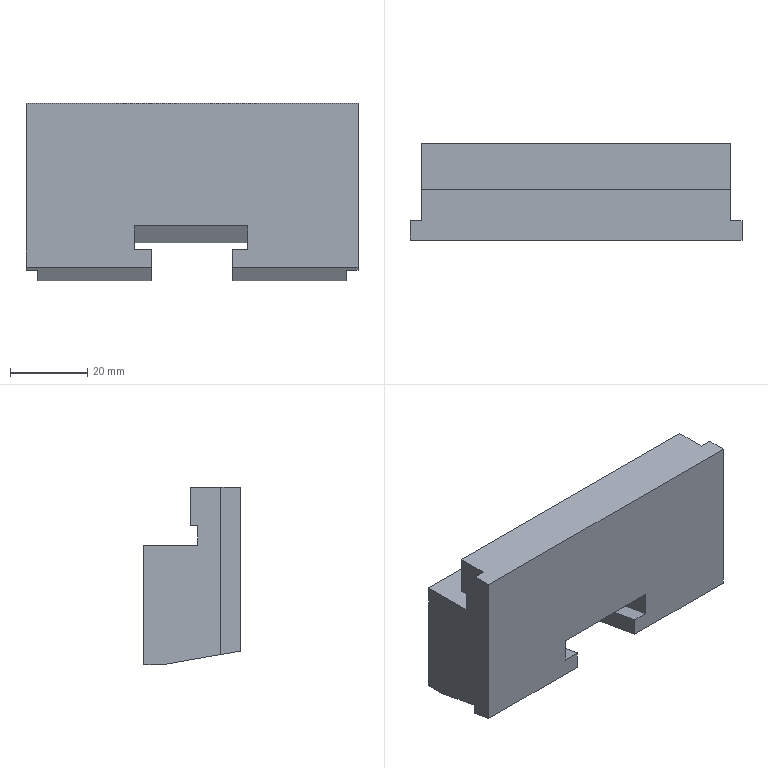Part | STEP file | 1 solid | 24 faces | box 86 x 25 x 46 mm | volume 68378 mm3 | plane 24